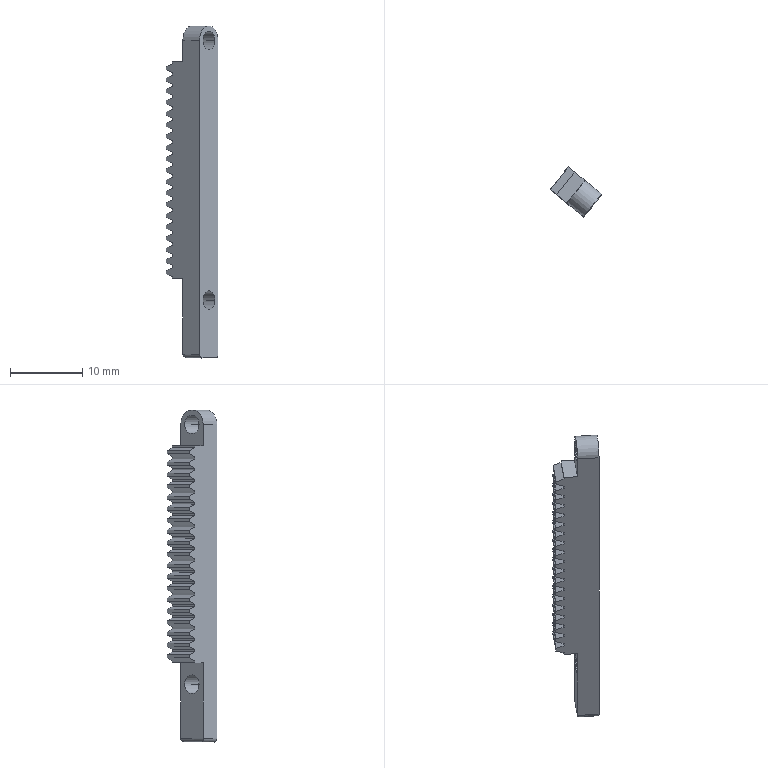Part | SolidWorks | features BaseBody 1 | 1 solid | 93 faces | box 7.179 x 6.889 x 46 mm | volume 810.413 mm3 | plane 85 | cylinder 8 | commonest cylinder face diameters 2.6 x4 1 x3 4 x1